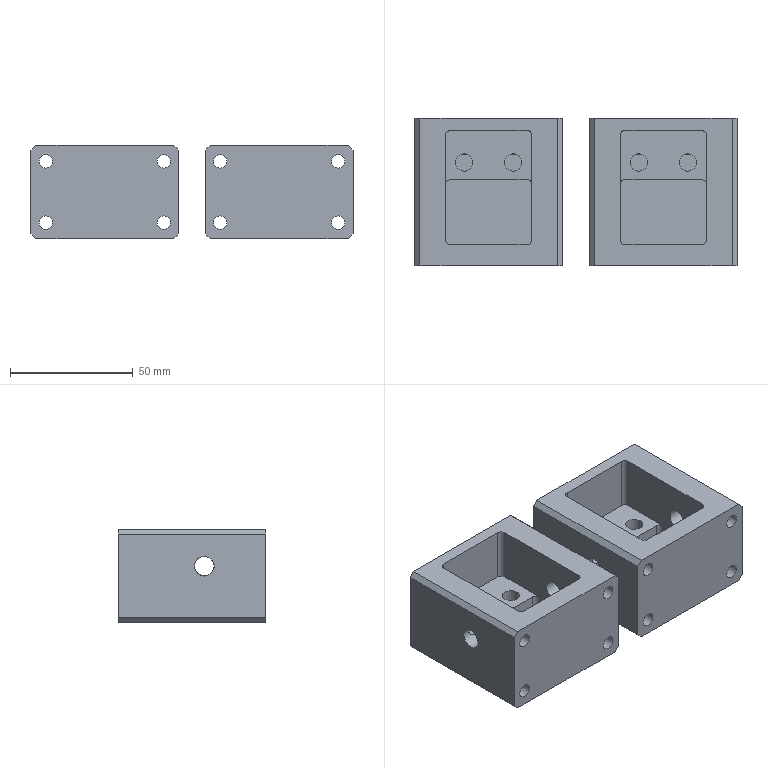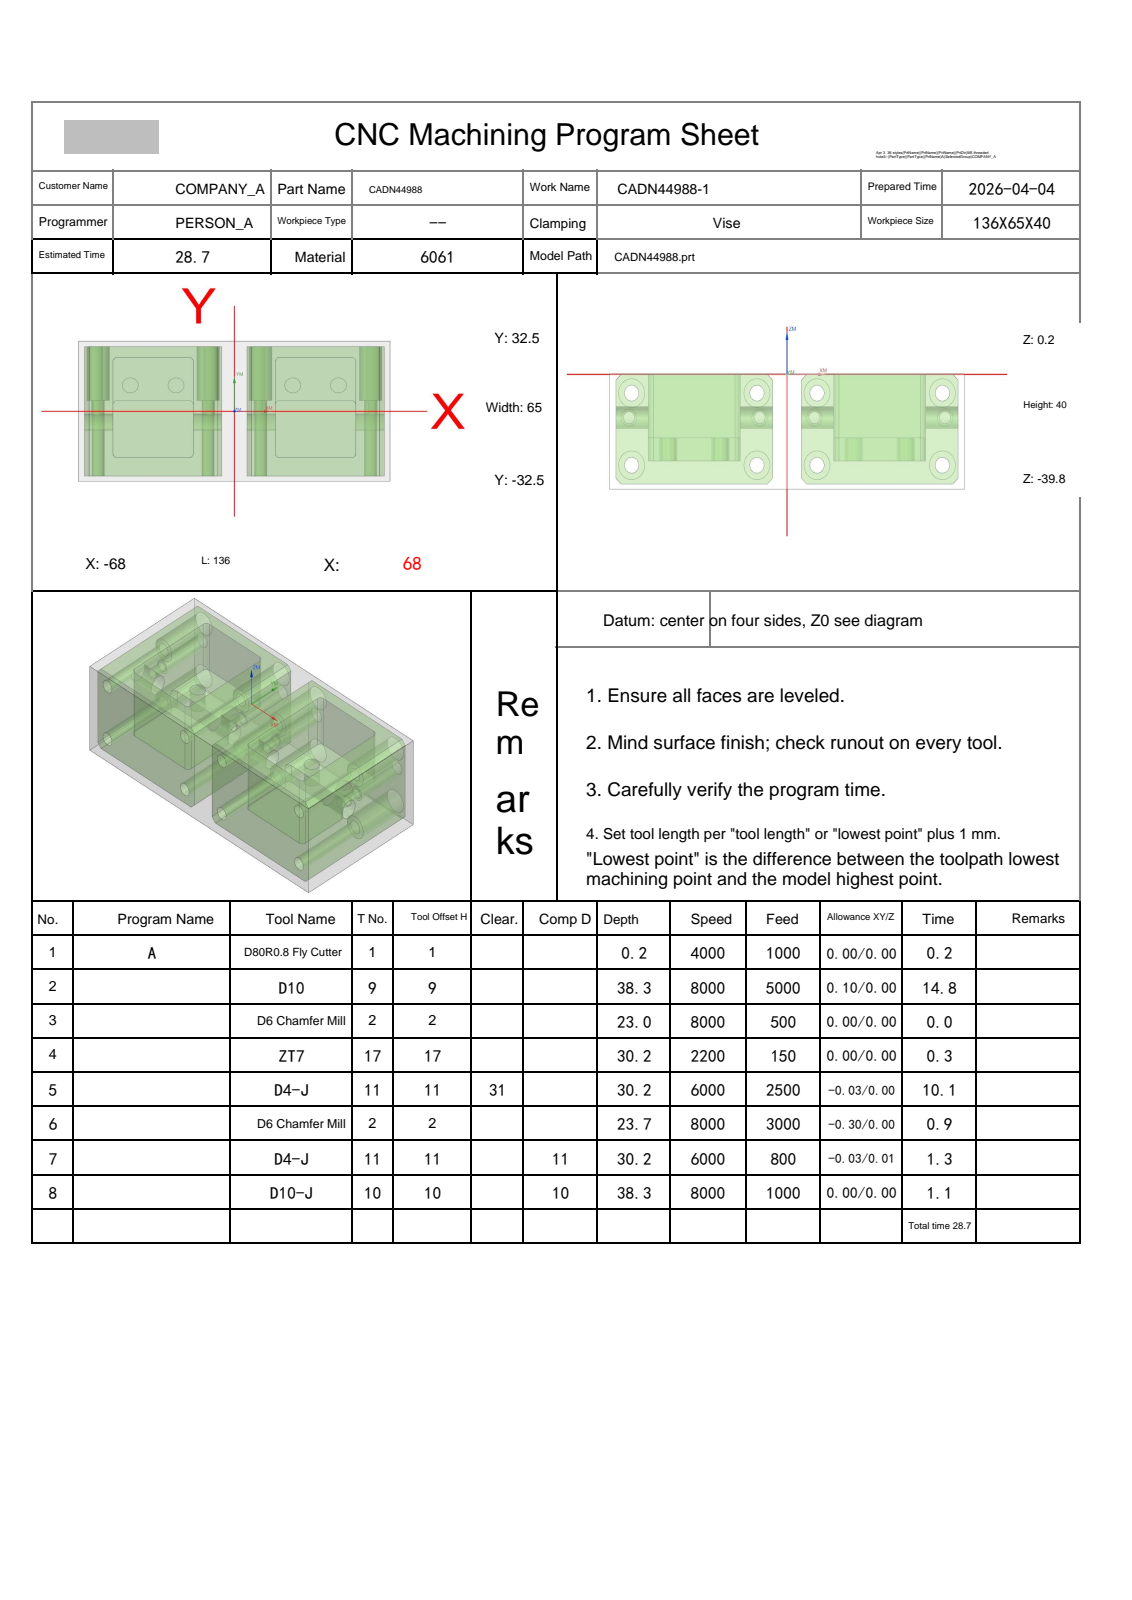NC program | NX | posted by the shop | part box 131 x 60 x 38 mm
Lines 1 to 32 of 30516:
%
O0001
(Machine time: 30.08 MIN)
(===Total Tool:6===)
(T1=D80R0.8 Fly Cutter D=80.  R=0.8  D-  H01 Z=0.    )
(T9=D10     D=10.  R=0.   D-  H09 Z=-38.1 )
(T2=D6 Chamfer Mill   D=6.   R=0.   D-  H02 Z=-23.5 )
(T17=ZT7    D=7.   DR_a=118 D-  H17 Z=-30.  )
(T11=D4-J   D=4.   R=0.   D11 H11 Z=-30.  )
(T10=D10-J  D=10.  R=0.   D10 H10 Z=-38.1 )
G80 G90 G17 G49 G40
G91 G28 Z0
M01
N1 T01 M06
(D80R0.8 Fly Cutter  D=80. R=0.8 H=01 ce=0.00 di=0.00)
G00 G90 G54 X-110.5 Y0.0 M03 S4000
G43 H01 Z20.
M08
Z2.
G01 Z0.0 F1000.
X-105.5
X105.5
X110.5
Z2.
G00 Z20.
G91 G28 Z0.0
M05
M09
G91 G28 Z0.0
M01